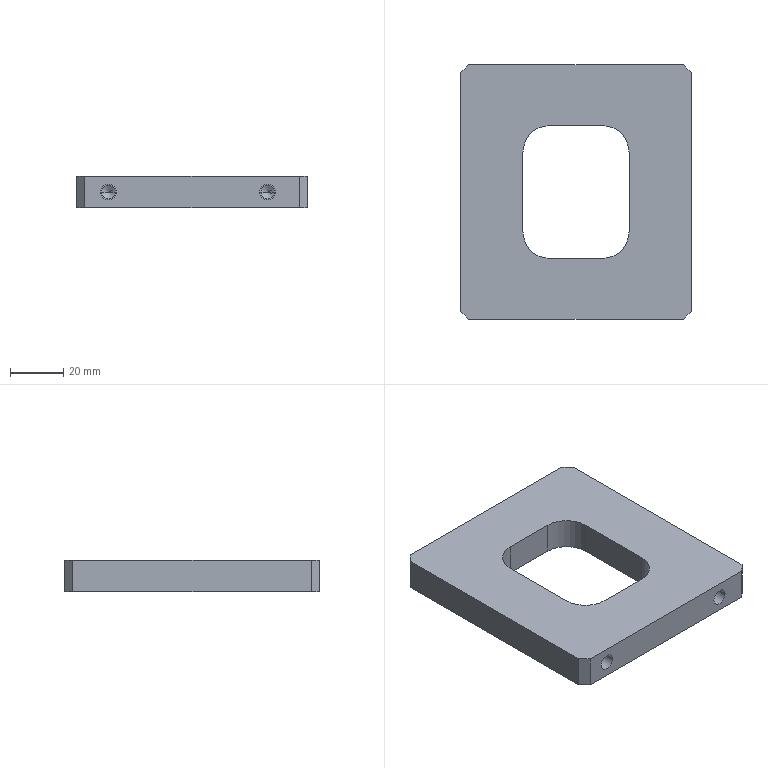Part | STEP file | J454-EBZ05-04-00-Part-1 | 1 solid | 60 faces | box 87 x 96 x 12 mm | volume 74063 mm3 | cylinder 28 | plane 20 | cone 12 | commonest cylinder face diameters 5.1 x12 6 x12 20 x4